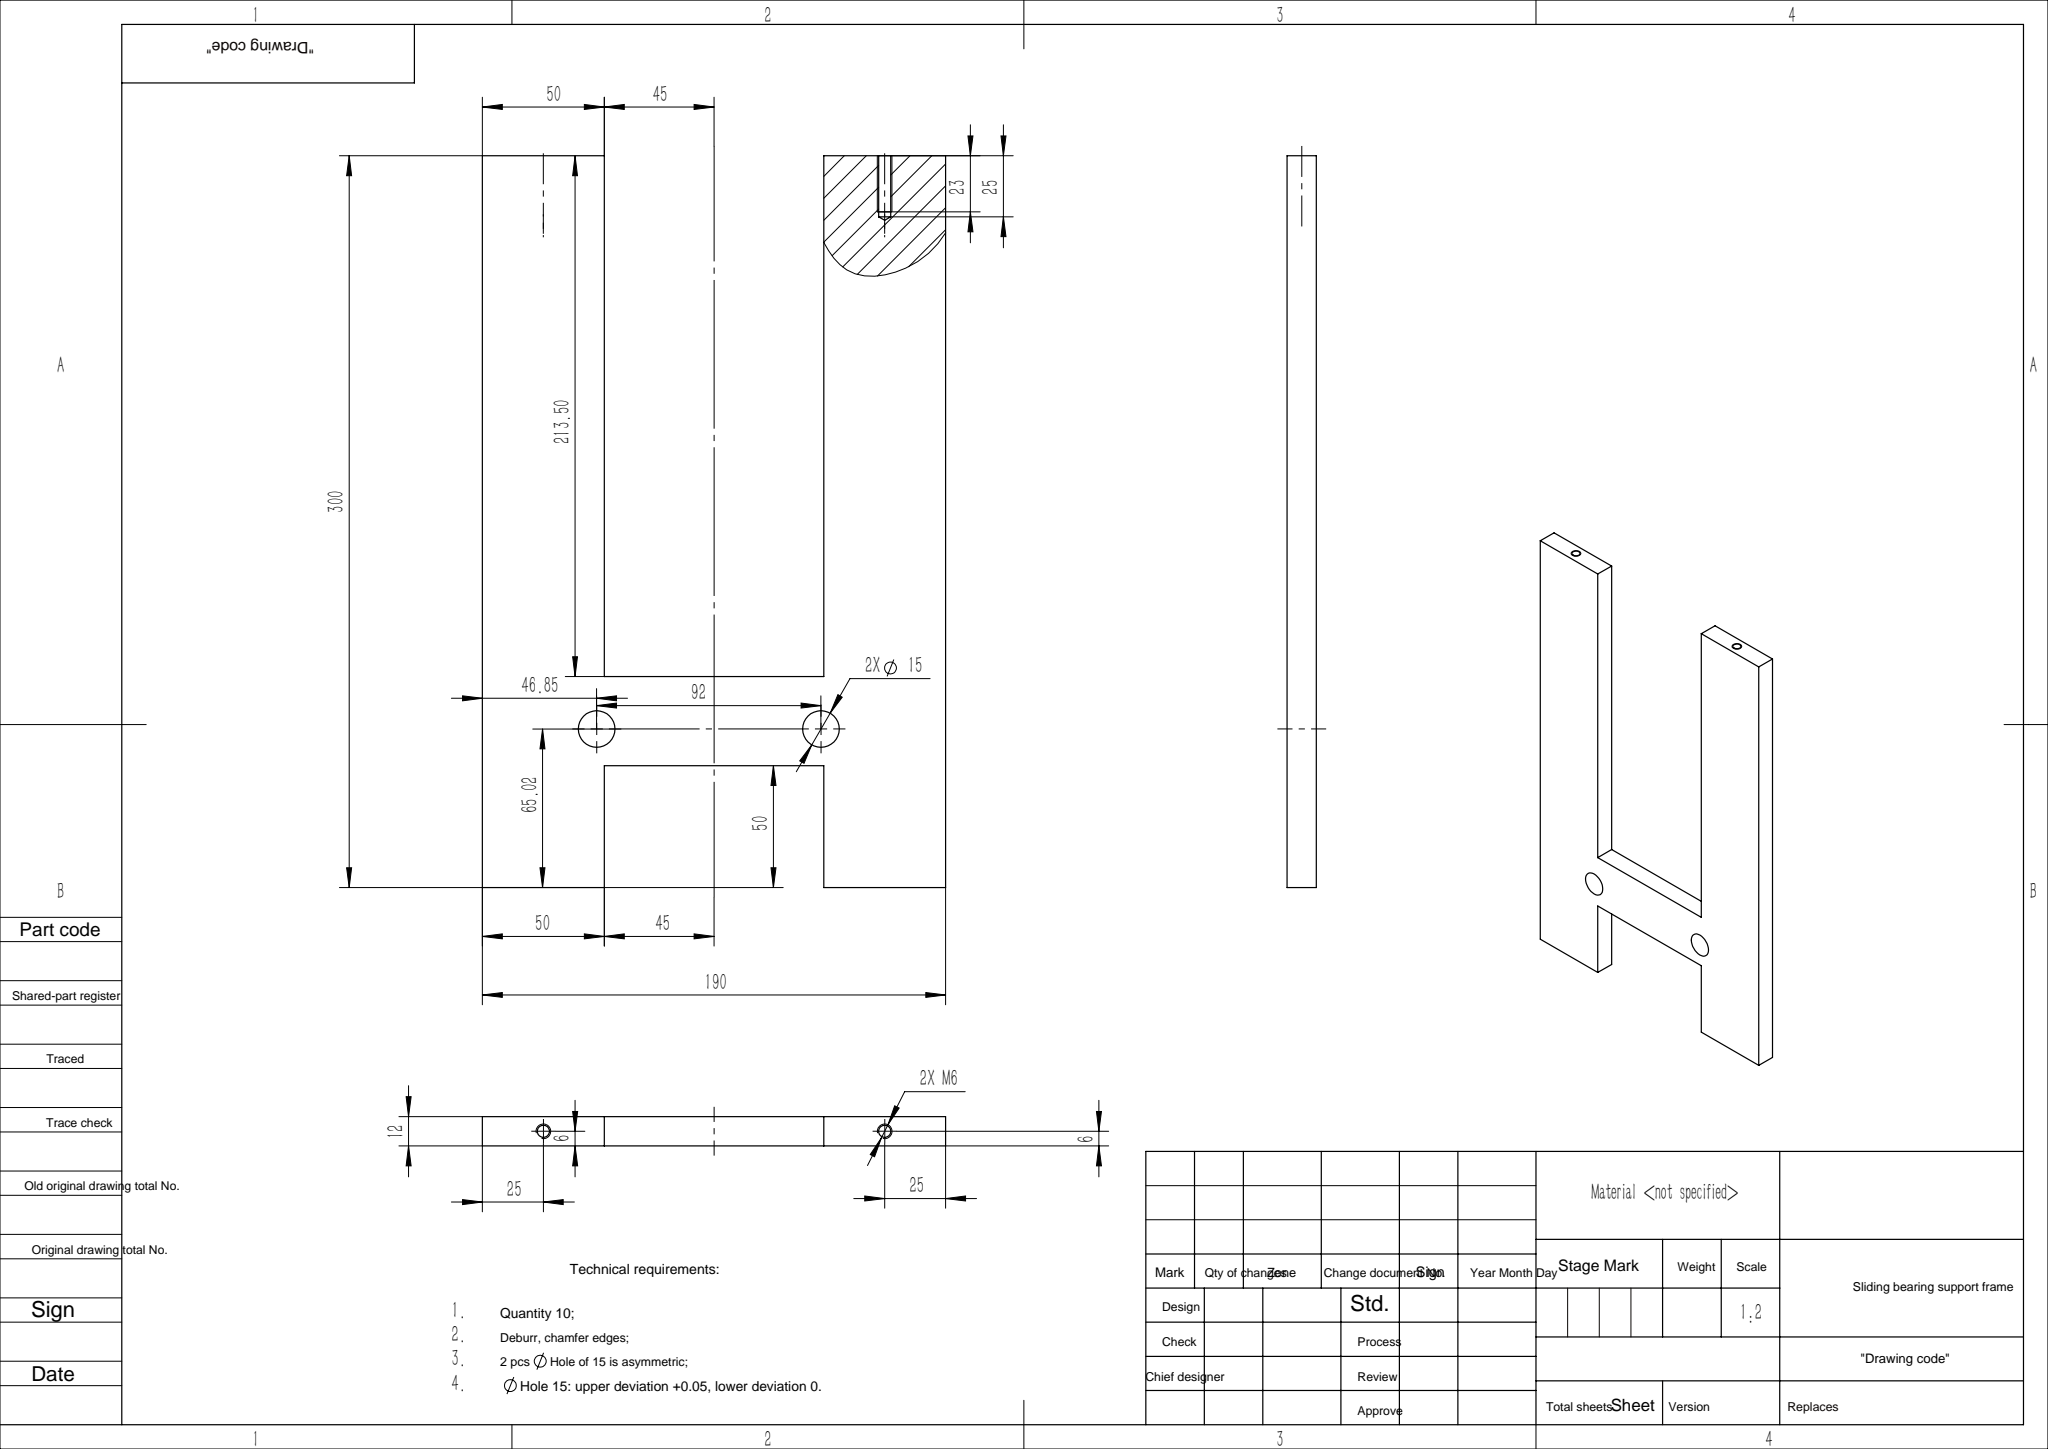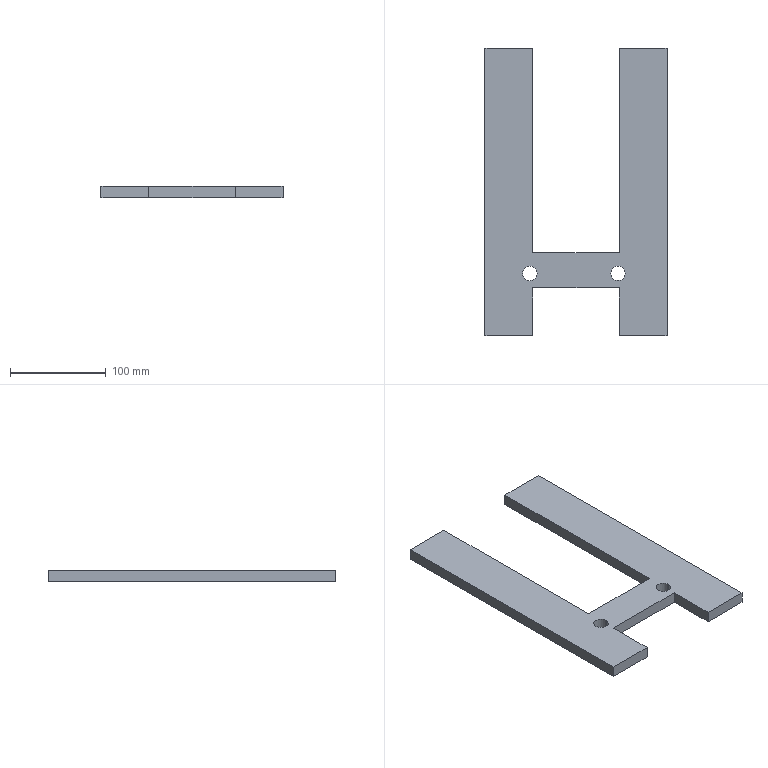Part | SolidWorks | features Extrusion 1, HoleWzd 1 | 1 solid | 26 faces | box 190 x 300 x 12 mm | volume 394178 mm3 | plane 14 | cylinder 8 | cone 4 | commonest cylinder face diameters 5 x4 15 x4
STEP:
#1=CARTESIAN_POINT('',(672.086,1780.,-467.5));
#2=VERTEX_POINT('',#1);
#3=CARTESIAN_POINT('',(672.086,1780.,-462.5));
#4=VERTEX_POINT('',#3);
#5=CARTESIAN_POINT('',(672.086,1780.,-465.));
#6=DIRECTION('',(0.,1.,0.));
#7=DIRECTION('',(0.,0.,1.));
#8=AXIS2_PLACEMENT_3D('',#5,#6,#7);
#9=CIRCLE('',#8,2.5);
#10=EDGE_CURVE('',#2,#4,#9,.T.);
#11=ORIENTED_EDGE('',*,*,#10,.F.);
#12=CARTESIAN_POINT('',(672.086,1805.,-467.5));
#13=VERTEX_POINT('',#12);
#14=CARTESIAN_POINT('',(672.086,1805.,-467.5));
#15=DIRECTION('',(0.,1.,0.));
#16=VECTOR('',#15,1000.);
#17=LINE('',#14,#16);
#18=EDGE_CURVE('',#2,#13,#17,.T.);
#19=ORIENTED_EDGE('',*,*,#18,.T.);
#20=CARTESIAN_POINT('',(672.086,1805.,-462.5));
#21=VERTEX_POINT('',#20);
#22=CARTESIAN_POINT('',(672.086,1805.,-465.));
#23=DIRECTION('',(0.,1.,0.));
#24=DIRECTION('',(0.,0.,1.));
#25=AXIS2_PLACEMENT_3D('',#22,#23,#24);
#26=CIRCLE('',#25,2.5);
#27=EDGE_CURVE('',#13,#21,#26,.T.);
#28=ORIENTED_EDGE('',*,*,#27,.T.);
#29=CARTESIAN_POINT('',(672.086,1805.,-462.5));
#30=DIRECTION('',(0.,1.,0.));
#31=VECTOR('',#30,1000.);
#32=LINE('',#29,#31);
#33=EDGE_CURVE('',#4,#21,#32,.T.);
#34=ORIENTED_EDGE('',*,*,#33,.F.);
#35=EDGE_LOOP('',(#11,#19,#28,#34));
#36=FACE_OUTER_BOUND('',#35,.T.);
#37=CARTESIAN_POINT('',(672.086,1805.,-465.));
#38=DIRECTION('',(0.,1.,0.));
#39=DIRECTION('',(0.,0.,1.));
#40=AXIS2_PLACEMENT_3D('',#37,#38,#39);
#41=CYLINDRICAL_SURFACE('',#40,2.5);
#42=ADVANCED_FACE('',(#36),#41,.F.);
#43=CARTESIAN_POINT('',(672.086,1778.557,-465.));
#44=VERTEX_POINT('',#43);
#45=CARTESIAN_POINT('',(672.086,1780.,-462.5));
#46=DIRECTION('',(0.,0.5,0.866));
#47=VECTOR('',#46,1000.);
#48=LINE('',#45,#47);
#49=EDGE_CURVE('',#44,#4,#48,.T.);
#50=ORIENTED_EDGE('',*,*,#49,.F.);
#51=CARTESIAN_POINT('',(672.086,1780.,-467.5));
#52=DIRECTION('',(0.,0.5,-0.866));
#53=VECTOR('',#52,1000.);
#54=LINE('',#51,#53);
#55=EDGE_CURVE('',#44,#2,#54,.T.);
#56=ORIENTED_EDGE('',*,*,#55,.T.);
#57=ORIENTED_EDGE('',*,*,#10,.T.);
#58=EDGE_LOOP('',(#50,#56,#57));
#59=FACE_OUTER_BOUND('',#58,.T.);
#60=CARTESIAN_POINT('',(672.086,1780.,-465.));
#61=DIRECTION('',(0.,1.,0.));
#62=DIRECTION('',(0.,0.,1.));
#63=AXIS2_PLACEMENT_3D('',#60,#61,#62);
#64=CONICAL_SURFACE('',#63,2.5,1.047);
#65=ADVANCED_FACE('',(#59),#64,.F.);
#66=CARTESIAN_POINT('',(532.086,1780.,-467.5));
#67=VERTEX_POINT('',#66);
#68=CARTESIAN_POINT('',(532.086,1780.,-462.5));
#69=VERTEX_POINT('',#68);
#70=CARTESIAN_POINT('',(532.086,1780.,-465.));
#71=DIRECTION('',(0.,1.,0.));
#72=DIRECTION('',(0.,0.,1.));
#73=AXIS2_PLACEMENT_3D('',#70,#71,#72);
#74=CIRCLE('',#73,2.5);
#75=EDGE_CURVE('',#67,#69,#74,.T.);
#76=ORIENTED_EDGE('',*,*,#75,.F.);
#77=CARTESIAN_POINT('',(532.086,1805.,-467.5));
#78=VERTEX_POINT('',#77);
#79=CARTESIAN_POINT('',(532.086,1805.,-467.5));
#80=DIRECTION('',(0.,1.,0.));
#81=VECTOR('',#80,1000.);
#82=LINE('',#79,#81);
#83=EDGE_CURVE('',#67,#78,#82,.T.);
#84=ORIENTED_EDGE('',*,*,#83,.T.);
#85=CARTESIAN_POINT('',(532.086,1805.,-462.5));
#86=VERTEX_POINT('',#85);
#87=CARTESIAN_POINT('',(532.086,1805.,-465.));
#88=DIRECTION('',(0.,1.,0.));
#89=DIRECTION('',(0.,0.,1.));
#90=AXIS2_PLACEMENT_3D('',#87,#88,#89);
#91=CIRCLE('',#90,2.5);
#92=EDGE_CURVE('',#78,#86,#91,.T.);
#93=ORIENTED_EDGE('',*,*,#92,.T.);
#94=CARTESIAN_POINT('',(532.086,1805.,-462.5));
#95=DIRECTION('',(0.,1.,0.));
#96=VECTOR('',#95,1000.);
#97=LINE('',#94,#96);
#98=EDGE_CURVE('',#69,#86,#97,.T.);
#99=ORIENTED_EDGE('',*,*,#98,.F.);
#100=EDGE_LOOP('',(#76,#84,#93,#99));
#101=FACE_OUTER_BOUND('',#100,.T.);
#102=CARTESIAN_POINT('',(532.086,1805.,-465.));
#103=DIRECTION('',(0.,1.,0.));
#104=DIRECTION('',(0.,0.,1.));
#105=AXIS2_PLACEMENT_3D('',#102,#103,#104);
#106=CYLINDRICAL_SURFACE('',#105,2.5);
#107=ADVANCED_FACE('',(#101),#106,.F.);
#108=CARTESIAN_POINT('',(532.086,1778.557,-465.));
#109=VERTEX_POINT('',#108);
#110=CARTESIAN_POINT('',(532.086,1780.,-462.5));
#111=DIRECTION('',(0.,0.5,0.866));
#112=VECTOR('',#111,1000.);
#113=LINE('',#110,#112);
#114=EDGE_CURVE('',#109,#69,#113,.T.);
#115=ORIENTED_EDGE('',*,*,#114,.F.);
#116=CARTESIAN_POINT('',(532.086,1780.,-467.5));
#117=DIRECTION('',(0.,0.5,-0.866));
#118=VECTOR('',#117,1000.);
#119=LINE('',#116,#118);
#120=EDGE_CURVE('',#109,#67,#119,.T.);
#121=ORIENTED_EDGE('',*,*,#120,.T.);
#122=ORIENTED_EDGE('',*,*,#75,.T.);
#123=EDGE_LOOP('',(#115,#121,#122));
#124=FACE_OUTER_BOUND('',#123,.T.);
#125=CARTESIAN_POINT('',(532.086,1780.,-465.));
#126=DIRECTION('',(0.,1.,0.));
#127=DIRECTION('',(0.,0.,1.));
#128=AXIS2_PLACEMENT_3D('',#125,#126,#127);
#129=CONICAL_SURFACE('',#128,2.5,1.047);
#130=ADVANCED_FACE('',(#124),#129,.F.);
#131=CARTESIAN_POINT('',(653.439,1570.019,-471.));
#132=VERTEX_POINT('',#131);
#133=CARTESIAN_POINT('',(638.439,1570.019,-471.));
#134=VERTEX_POINT('',#133);
#135=CARTESIAN_POINT('',(645.939,1570.019,-471.));
#136=DIRECTION('',(0.,0.,-1.));
#137=DIRECTION('',(-1.,0.,0.));
#138=AXIS2_PLACEMENT_3D('',#135,#136,#137);
#139=CIRCLE('',#138,7.5);
#140=EDGE_CURVE('',#132,#134,#139,.T.);
#141=ORIENTED_EDGE('',*,*,#140,.T.);
#142=CARTESIAN_POINT('',(638.439,1570.019,-459.));
#143=VERTEX_POINT('',#142);
#144=CARTESIAN_POINT('',(638.439,1570.019,-471.));
#145=DIRECTION('',(0.,0.,1.));
#146=VECTOR('',#145,1000.);
#147=LINE('',#144,#146);
#148=EDGE_CURVE('',#134,#143,#147,.T.);
#149=ORIENTED_EDGE('',*,*,#148,.T.);
#150=CARTESIAN_POINT('',(653.439,1570.019,-459.));
#151=VERTEX_POINT('',#150);
#152=CARTESIAN_POINT('',(645.939,1570.019,-459.));
#153=DIRECTION('',(0.,0.,-1.));
#154=DIRECTION('',(-1.,0.,0.));
#155=AXIS2_PLACEMENT_3D('',#152,#153,#154);
#156=CIRCLE('',#155,7.5);
#157=EDGE_CURVE('',#151,#143,#156,.T.);
#158=ORIENTED_EDGE('',*,*,#157,.F.);
#159=CARTESIAN_POINT('',(653.439,1570.019,-471.));
#160=DIRECTION('',(0.,0.,1.));
#161=VECTOR('',#160,1000.);
#162=LINE('',#159,#161);
#163=EDGE_CURVE('',#132,#151,#162,.T.);
#164=ORIENTED_EDGE('',*,*,#163,.F.);
#165=EDGE_LOOP('',(#141,#149,#158,#164));
#166=FACE_OUTER_BOUND('',#165,.T.);
#167=CARTESIAN_POINT('',(645.939,1570.019,-471.));
#168=DIRECTION('',(0.,0.,1.));
#169=DIRECTION('',(1.,0.,0.));
#170=AXIS2_PLACEMENT_3D('',#167,#168,#169);
#171=CYLINDRICAL_SURFACE('',#170,7.5);
#172=ADVANCED_FACE('',(#166),#171,.F.);
#173=CARTESIAN_POINT('',(561.439,1570.019,-471.));
#174=VERTEX_POINT('',#173);
#175=CARTESIAN_POINT('',(546.439,1570.019,-471.));
#176=VERTEX_POINT('',#175);
#177=CARTESIAN_POINT('',(553.939,1570.019,-471.));
#178=DIRECTION('',(0.,0.,-1.));
#179=DIRECTION('',(-1.,0.,0.));
#180=AXIS2_PLACEMENT_3D('',#177,#178,#179);
#181=CIRCLE('',#180,7.5);
#182=EDGE_CURVE('',#174,#176,#181,.T.);
#183=ORIENTED_EDGE('',*,*,#182,.T.);
#184=CARTESIAN_POINT('',(546.439,1570.019,-459.));
#185=VERTEX_POINT('',#184);
#186=CARTESIAN_POINT('',(546.439,1570.019,-471.));
#187=DIRECTION('',(0.,0.,1.));
#188=VECTOR('',#187,1000.);
#189=LINE('',#186,#188);
#190=EDGE_CURVE('',#176,#185,#189,.T.);
#191=ORIENTED_EDGE('',*,*,#190,.T.);
#192=CARTESIAN_POINT('',(561.439,1570.019,-459.));
#193=VERTEX_POINT('',#192);
#194=CARTESIAN_POINT('',(553.939,1570.019,-459.));
#195=DIRECTION('',(0.,0.,-1.));
#196=DIRECTION('',(-1.,0.,0.));
#197=AXIS2_PLACEMENT_3D('',#194,#195,#196);
#198=CIRCLE('',#197,7.5);
#199=EDGE_CURVE('',#193,#185,#198,.T.);
#200=ORIENTED_EDGE('',*,*,#199,.F.);
#201=CARTESIAN_POINT('',(561.439,1570.019,-471.));
#202=DIRECTION('',(0.,0.,1.));
#203=VECTOR('',#202,1000.);
#204=LINE('',#201,#203);
#205=EDGE_CURVE('',#174,#193,#204,.T.);
#206=ORIENTED_EDGE('',*,*,#205,.F.);
#207=EDGE_LOOP('',(#183,#191,#200,#206));
#208=FACE_OUTER_BOUND('',#207,.T.);
#209=CARTESIAN_POINT('',(553.939,1570.019,-471.));
#210=DIRECTION('',(0.,0.,1.));
#211=DIRECTION('',(1.,0.,0.));
#212=AXIS2_PLACEMENT_3D('',#209,#210,#211);
#213=CYLINDRICAL_SURFACE('',#212,7.5);
#214=ADVANCED_FACE('',(#208),#213,.F.);
#215=ORIENTED_EDGE('',*,*,#182,.F.);
#216=CARTESIAN_POINT('',(553.939,1570.019,-471.));
#217=DIRECTION('',(0.,0.,-1.));
#218=DIRECTION('',(-1.,0.,0.));
#219=AXIS2_PLACEMENT_3D('',#216,#217,#218);
#220=CIRCLE('',#219,7.5);
#221=EDGE_CURVE('',#176,#174,#220,.T.);
#222=ORIENTED_EDGE('',*,*,#221,.F.);
#223=EDGE_LOOP('',(#215,#222));
#224=FACE_BOUND('',#223,.T.);
#225=CARTESIAN_POINT('',(507.086,1805.,-471.));
#226=VERTEX_POINT('',#225);
#227=CARTESIAN_POINT('',(557.086,1805.,-471.));
#228=VERTEX_POINT('',#227);
#229=CARTESIAN_POINT('',(557.086,1805.,-471.));
#230=DIRECTION('',(1.,0.,0.));
#231=VECTOR('',#230,1000.);
#232=LINE('',#229,#231);
#233=EDGE_CURVE('',#226,#228,#232,.T.);
#234=ORIENTED_EDGE('',*,*,#233,.T.);
#235=CARTESIAN_POINT('',(557.086,1591.5,-471.));
#236=VERTEX_POINT('',#235);
#237=CARTESIAN_POINT('',(557.086,1805.,-471.));
#238=DIRECTION('',(0.,-1.,0.));
#239=VECTOR('',#238,1000.);
#240=LINE('',#237,#239);
#241=EDGE_CURVE('',#228,#236,#240,.T.);
#242=ORIENTED_EDGE('',*,*,#241,.T.);
#243=CARTESIAN_POINT('',(647.086,1591.5,-471.));
#244=VERTEX_POINT('',#243);
#245=CARTESIAN_POINT('',(557.086,1591.5,-471.));
#246=DIRECTION('',(1.,0.,0.));
#247=VECTOR('',#246,1000.);
#248=LINE('',#245,#247);
#249=EDGE_CURVE('',#236,#244,#248,.T.);
#250=ORIENTED_EDGE('',*,*,#249,.T.);
#251=CARTESIAN_POINT('',(647.086,1805.,-471.));
#252=VERTEX_POINT('',#251);
#253=CARTESIAN_POINT('',(647.086,1805.,-471.));
#254=DIRECTION('',(0.,1.,0.));
#255=VECTOR('',#254,1000.);
#256=LINE('',#253,#255);
#257=EDGE_CURVE('',#244,#252,#256,.T.);
#258=ORIENTED_EDGE('',*,*,#257,.T.);
#259=CARTESIAN_POINT('',(697.086,1805.,-471.));
#260=VERTEX_POINT('',#259);
#261=CARTESIAN_POINT('',(647.086,1805.,-471.));
#262=DIRECTION('',(1.,0.,0.));
#263=VECTOR('',#262,1000.);
#264=LINE('',#261,#263);
#265=EDGE_CURVE('',#252,#260,#264,.T.);
#266=ORIENTED_EDGE('',*,*,#265,.T.);
#267=CARTESIAN_POINT('',(697.086,1505.,-471.));
#268=VERTEX_POINT('',#267);
#269=CARTESIAN_POINT('',(697.086,1805.,-471.));
#270=DIRECTION('',(0.,-1.,0.));
#271=VECTOR('',#270,1000.);
#272=LINE('',#269,#271);
#273=EDGE_CURVE('',#260,#268,#272,.T.);
#274=ORIENTED_EDGE('',*,*,#273,.T.);
#275=CARTESIAN_POINT('',(647.086,1505.,-471.));
#276=VERTEX_POINT('',#275);
#277=CARTESIAN_POINT('',(697.086,1505.,-471.));
#278=DIRECTION('',(-1.,0.,0.));
#279=VECTOR('',#278,1000.);
#280=LINE('',#277,#279);
#281=EDGE_CURVE('',#268,#276,#280,.T.);
#282=ORIENTED_EDGE('',*,*,#281,.T.);
#283=CARTESIAN_POINT('',(647.086,1555.,-471.));
#284=VERTEX_POINT('',#283);
#285=CARTESIAN_POINT('',(647.086,1555.,-471.));
#286=DIRECTION('',(0.,1.,0.));
#287=VECTOR('',#286,1000.);
#288=LINE('',#285,#287);
#289=EDGE_CURVE('',#276,#284,#288,.T.);
#290=ORIENTED_EDGE('',*,*,#289,.T.);
#291=CARTESIAN_POINT('',(557.086,1555.,-471.));
#292=VERTEX_POINT('',#291);
#293=CARTESIAN_POINT('',(647.086,1555.,-471.));
#294=DIRECTION('',(-1.,0.,0.));
#295=VECTOR('',#294,1000.);
#296=LINE('',#293,#295);
#297=EDGE_CURVE('',#284,#292,#296,.T.);
#298=ORIENTED_EDGE('',*,*,#297,.T.);
#299=CARTESIAN_POINT('',(557.086,1505.,-471.));
#300=VERTEX_POINT('',#299);
#301=CARTESIAN_POINT('',(557.086,1555.,-471.));
#302=DIRECTION('',(0.,-1.,0.));
#303=VECTOR('',#302,1000.);
#304=LINE('',#301,#303);
#305=EDGE_CURVE('',#292,#300,#304,.T.);
#306=ORIENTED_EDGE('',*,*,#305,.T.);
#307=CARTESIAN_POINT('',(507.086,1505.,-471.));
#308=VERTEX_POINT('',#307);
#309=CARTESIAN_POINT('',(507.086,1505.,-471.));
#310=DIRECTION('',(-1.,0.,0.));
#311=VECTOR('',#310,1000.);
#312=LINE('',#309,#311);
#313=EDGE_CURVE('',#300,#308,#312,.T.);
#314=ORIENTED_EDGE('',*,*,#313,.T.);
#315=CARTESIAN_POINT('',(507.086,1805.,-471.));
#316=DIRECTION('',(0.,1.,0.));
#317=VECTOR('',#316,1000.);
#318=LINE('',#315,#317);
#319=EDGE_CURVE('',#308,#226,#318,.T.);
#320=ORIENTED_EDGE('',*,*,#319,.T.);
#321=EDGE_LOOP('',(#234,#242,#250,#258,#266,#274,#282,#290,#298,#306,#314,#320));
#322=FACE_OUTER_BOUND('',#321,.T.);
#323=ORIENTED_EDGE('',*,*,#140,.F.);
#324=CARTESIAN_POINT('',(645.939,1570.019,-471.));
#325=DIRECTION('',(0.,0.,-1.));
#326=DIRECTION('',(-1.,0.,0.));
#327=AXIS2_PLACEMENT_3D('',#324,#325,#326);
#328=CIRCLE('',#327,7.5);
#329=EDGE_CURVE('',#134,#132,#328,.T.);
#330=ORIENTED_EDGE('',*,*,#329,.F.);
#331=EDGE_LOOP('',(#323,#330));
#332=FACE_BOUND('',#331,.T.);
#333=CARTESIAN_POINT('',(0.,0.,-471.));
#334=DIRECTION('',(0.,0.,1.));
#335=DIRECTION('',(1.,0.,0.));
#336=AXIS2_PLACEMENT_3D('',#333,#334,#335);
#337=PLANE('',#336);
#338=ADVANCED_FACE('',(#224,#322,#332),#337,.F.);
#339=ORIENTED_EDGE('',*,*,#199,.T.);
#340=CARTESIAN_POINT('',(553.939,1570.019,-459.));
#341=DIRECTION('',(0.,0.,-1.));
#342=DIRECTION('',(-1.,0.,0.));
#343=AXIS2_PLACEMENT_3D('',#340,#341,#342);
#344=CIRCLE('',#343,7.5);
#345=EDGE_CURVE('',#185,#193,#344,.T.);
#346=ORIENTED_EDGE('',*,*,#345,.T.);
#347=EDGE_LOOP('',(#339,#346));
#348=FACE_BOUND('',#347,.T.);
#349=CARTESIAN_POINT('',(507.086,1805.,-459.));
#350=VERTEX_POINT('',#349);
#351=CARTESIAN_POINT('',(557.086,1805.,-459.));
#352=VERTEX_POINT('',#351);
#353=CARTESIAN_POINT('',(557.086,1805.,-459.));
#354=DIRECTION('',(1.,0.,0.));
#355=VECTOR('',#354,1000.);
#356=LINE('',#353,#355);
#357=EDGE_CURVE('',#350,#352,#356,.T.);
#358=ORIENTED_EDGE('',*,*,#357,.F.);
#359=CARTESIAN_POINT('',(507.086,1505.,-459.));
#360=VERTEX_POINT('',#359);
#361=CARTESIAN_POINT('',(507.086,1805.,-459.));
#362=DIRECTION('',(0.,1.,0.));
#363=VECTOR('',#362,1000.);
#364=LINE('',#361,#363);
#365=EDGE_CURVE('',#360,#350,#364,.T.);
#366=ORIENTED_EDGE('',*,*,#365,.F.);
#367=CARTESIAN_POINT('',(557.086,1505.,-459.));
#368=VERTEX_POINT('',#367);
#369=CARTESIAN_POINT('',(507.086,1505.,-459.));
#370=DIRECTION('',(-1.,0.,0.));
#371=VECTOR('',#370,1000.);
#372=LINE('',#369,#371);
#373=EDGE_CURVE('',#368,#360,#372,.T.);
#374=ORIENTED_EDGE('',*,*,#373,.F.);
#375=CARTESIAN_POINT('',(557.086,1555.,-459.));
#376=VERTEX_POINT('',#375);
#377=CARTESIAN_POINT('',(557.086,1555.,-459.));
#378=DIRECTION('',(0.,-1.,0.));
#379=VECTOR('',#378,1000.);
#380=LINE('',#377,#379);
#381=EDGE_CURVE('',#376,#368,#380,.T.);
#382=ORIENTED_EDGE('',*,*,#381,.F.);
#383=CARTESIAN_POINT('',(647.086,1555.,-459.));
#384=VERTEX_POINT('',#383);
#385=CARTESIAN_POINT('',(647.086,1555.,-459.));
#386=DIRECTION('',(-1.,0.,0.));
#387=VECTOR('',#386,1000.);
#388=LINE('',#385,#387);
#389=EDGE_CURVE('',#384,#376,#388,.T.);
#390=ORIENTED_EDGE('',*,*,#389,.F.);
#391=CARTESIAN_POINT('',(647.086,1505.,-459.));
#392=VERTEX_POINT('',#391);
#393=CARTESIAN_POINT('',(647.086,1555.,-459.));
#394=DIRECTION('',(0.,1.,0.));
#395=VECTOR('',#394,1000.);
#396=LINE('',#393,#395);
#397=EDGE_CURVE('',#392,#384,#396,.T.);
#398=ORIENTED_EDGE('',*,*,#397,.F.);
#399=CARTESIAN_POINT('',(697.086,1505.,-459.));
#400=VERTEX_POINT('',#399);
#401=CARTESIAN_POINT('',(697.086,1505.,-459.));
#402=DIRECTION('',(-1.,0.,0.));
#403=VECTOR('',#402,1000.);
#404=LINE('',#401,#403);
#405=EDGE_CURVE('',#400,#392,#404,.T.);
#406=ORIENTED_EDGE('',*,*,#405,.F.);
#407=CARTESIAN_POINT('',(697.086,1805.,-459.));
#408=VERTEX_POINT('',#407);
#409=CARTESIAN_POINT('',(697.086,1805.,-459.));
#410=DIRECTION('',(0.,-1.,0.));
#411=VECTOR('',#410,1000.);
#412=LINE('',#409,#411);
#413=EDGE_CURVE('',#408,#400,#412,.T.);
#414=ORIENTED_EDGE('',*,*,#413,.F.);
#415=CARTESIAN_POINT('',(647.086,1805.,-459.));
#416=VERTEX_POINT('',#415);
#417=CARTESIAN_POINT('',(647.086,1805.,-459.));
#418=DIRECTION('',(1.,0.,0.));
#419=VECTOR('',#418,1000.);
#420=LINE('',#417,#419);
#421=EDGE_CURVE('',#416,#408,#420,.T.);
#422=ORIENTED_EDGE('',*,*,#421,.F.);
#423=CARTESIAN_POINT('',(647.086,1591.5,-459.));
#424=VERTEX_POINT('',#423);
#425=CARTESIAN_POINT('',(647.086,1805.,-459.));
#426=DIRECTION('',(0.,1.,0.));
#427=VECTOR('',#426,1000.);
#428=LINE('',#425,#427);
#429=EDGE_CURVE('',#424,#416,#428,.T.);
#430=ORIENTED_EDGE('',*,*,#429,.F.);
#431=CARTESIAN_POINT('',(557.086,1591.5,-459.));
#432=VERTEX_POINT('',#431);
#433=CARTESIAN_POINT('',(557.086,1591.5,-459.));
#434=DIRECTION('',(1.,0.,0.));
#435=VECTOR('',#434,1000.);
#436=LINE('',#433,#435);
#437=EDGE_CURVE('',#432,#424,#436,.T.);
#438=ORIENTED_EDGE('',*,*,#437,.F.);
#439=CARTESIAN_POINT('',(557.086,1805.,-459.));
#440=DIRECTION('',(0.,-1.,0.));
#441=VECTOR('',#440,1000.);
#442=LINE('',#439,#441);
#443=EDGE_CURVE('',#352,#432,#442,.T.);
#444=ORIENTED_EDGE('',*,*,#443,.F.);
#445=EDGE_LOOP('',(#358,#366,#374,#382,#390,#398,#406,#414,#422,#430,#438,#444));
#446=FACE_OUTER_BOUND('',#445,.T.);
#447=ORIENTED_EDGE('',*,*,#157,.T.);
#448=CARTESIAN_POINT('',(645.939,1570.019,-459.));
#449=DIRECTION('',(0.,0.,-1.));
#450=DIRECTION('',(-1.,0.,0.));
#451=AXIS2_PLACEMENT_3D('',#448,#449,#450);
#452=CIRCLE('',#451,7.5);
#453=EDGE_CURVE('',#143,#151,#452,.T.);
#454=ORIENTED_EDGE('',*,*,#453,.T.);
#455=EDGE_LOOP('',(#447,#454));
#456=FACE_BOUND('',#455,.T.);
#457=CARTESIAN_POINT('',(0.,0.,-459.));
#458=DIRECTION('',(0.,0.,1.));
#459=DIRECTION('',(1.,0.,0.));
#460=AXIS2_PLACEMENT_3D('',#457,#458,#459);
#461=PLANE('',#460);
#462=ADVANCED_FACE('',(#348,#446,#456),#461,.T.);
#463=CARTESIAN_POINT('',(532.086,1805.,-465.));
#464=DIRECTION('',(0.,1.,0.));
#465=DIRECTION('',(0.,0.,1.));
#466=AXIS2_PLACEMENT_3D('',#463,#464,#465);
#467=CIRCLE('',#466,2.5);
#468=EDGE_CURVE('',#86,#78,#467,.T.);
#469=ORIENTED_EDGE('',*,*,#468,.F.);
#470=ORIENTED_EDGE('',*,*,#92,.F.);
#471=EDGE_LOOP('',(#469,#470));
#472=FACE_BOUND('',#471,.T.);
#473=ORIENTED_EDGE('',*,*,#357,.T.);
#474=CARTESIAN_POINT('',(557.086,1805.,-471.));
#475=DIRECTION('',(0.,0.,1.));
#476=VECTOR('',#475,1000.);
#477=LINE('',#474,#476);
#478=EDGE_CURVE('',#228,#352,#477,.T.);
#479=ORIENTED_EDGE('',*,*,#478,.F.);
#480=ORIENTED_EDGE('',*,*,#233,.F.);
#481=CARTESIAN_POINT('',(507.086,1805.,-471.));
#482=DIRECTION('',(0.,0.,1.));
#483=VECTOR('',#482,1000.);
#484=LINE('',#481,#483);
#485=EDGE_CURVE('',#226,#350,#484,.T.);
#486=ORIENTED_EDGE('',*,*,#485,.T.);
#487=EDGE_LOOP('',(#473,#479,#480,#486));
#488=FACE_OUTER_BOUND('',#487,.T.);
#489=CARTESIAN_POINT('',(557.086,1805.,-471.));
#490=DIRECTION('',(0.,-1.,0.));
#491=DIRECTION('',(1.,0.,0.));
#492=AXIS2_PLACEMENT_3D('',#489,#490,#491);
#493=PLANE('',#492);
#494=ADVANCED_FACE('',(#472,#488),#493,.F.);
#495=ORIENTED_EDGE('',*,*,#443,.T.);
#496=CARTESIAN_POINT('',(557.086,1591.5,-471.));
#497=DIRECTION('',(0.,0.,1.));
#498=VECTOR('',#497,1000.);
#499=LINE('',#496,#498);
#500=EDGE_CURVE('',#236,#432,#499,.T.);
#501=ORIENTED_EDGE('',*,*,#500,.F.);
#502=ORIENTED_EDGE('',*,*,#241,.F.);
#503=ORIENTED_EDGE('',*,*,#478,.T.);
#504=EDGE_LOOP('',(#495,#501,#502,#503));
#505=FACE_OUTER_BOUND('',#504,.T.);
#506=CARTESIAN_POINT('',(557.086,1805.,-471.));
#507=DIRECTION('',(-1.,0.,0.));
#508=DIRECTION('',(0.,0.,1.));
#509=AXIS2_PLACEMENT_3D('',#506,#507,#508);
#510=PLANE('',#509);
#511=ADVANCED_FACE('',(#505),#510,.F.);
#512=ORIENTED_EDGE('',*,*,#437,.T.);
#513=CARTESIAN_POINT('',(647.086,1591.5,-471.));
#514=DIRECTION('',(0.,0.,1.));
#515=VECTOR('',#514,1000.);
#516=LINE('',#513,#515);
#517=EDGE_CURVE('',#244,#424,#516,.T.);
#518=ORIENTED_EDGE('',*,*,#517,.F.);
#519=ORIENTED_EDGE('',*,*,#249,.F.);
#520=ORIENTED_EDGE('',*,*,#500,.T.);
#521=EDGE_LOOP('',(#512,#518,#519,#520));
#522=FACE_OUTER_BOUND('',#521,.T.);
#523=CARTESIAN_POINT('',(557.086,1591.5,-471.));
#524=DIRECTION('',(0.,-1.,0.));
#525=DIRECTION('',(0.,0.,-1.));
#526=AXIS2_PLACEMENT_3D('',#523,#524,#525);
#527=PLANE('',#526);
#528=ADVANCED_FACE('',(#522),#527,.F.);
#529=ORIENTED_EDGE('',*,*,#429,.T.);
#530=CARTESIAN_POINT('',(647.086,1805.,-471.));
#531=DIRECTION('',(0.,0.,1.));
#532=VECTOR('',#531,1000.);
#533=LINE('',#530,#532);
#534=EDGE_CURVE('',#252,#416,#533,.T.);
#535=ORIENTED_EDGE('',*,*,#534,.F.);
#536=ORIENTED_EDGE('',*,*,#257,.F.);
#537=ORIENTED_EDGE('',*,*,#517,.T.);
#538=EDGE_LOOP('',(#529,#535,#536,#537));
#539=FACE_OUTER_BOUND('',#538,.T.);
#540=CARTESIAN_POINT('',(647.086,1805.,-471.));
#541=DIRECTION('',(1.,0.,0.));
#542=DIRECTION('',(0.,0.,-1.));
#543=AXIS2_PLACEMENT_3D('',#540,#541,#542);
#544=PLANE('',#543);
#545=ADVANCED_FACE('',(#539),#544,.F.);
#546=CARTESIAN_POINT('',(672.086,1805.,-465.));
#547=DIRECTION('',(0.,1.,0.));
#548=DIRECTION('',(0.,0.,1.));
#549=AXIS2_PLACEMENT_3D('',#546,#547,#548);
#550=CIRCLE('',#549,2.5);
#551=EDGE_CURVE('',#21,#13,#550,.T.);
#552=ORIENTED_EDGE('',*,*,#551,.F.);
#553=ORIENTED_EDGE('',*,*,#27,.F.);
#554=EDGE_LOOP('',(#552,#553));
#555=FACE_BOUND('',#554,.T.);
#556=ORIENTED_EDGE('',*,*,#421,.T.);
#557=CARTESIAN_POINT('',(697.086,1805.,-471.));
#558=DIRECTION('',(0.,0.,1.));
#559=VECTOR('',#558,1000.);
#560=LINE('',#557,#559);
#561=EDGE_CURVE('',#260,#408,#560,.T.);
#562=ORIENTED_EDGE('',*,*,#561,.F.);
#563=ORIENTED_EDGE('',*,*,#265,.F.);
#564=ORIENTED_EDGE('',*,*,#534,.T.);
#565=EDGE_LOOP('',(#556,#562,#563,#564));
#566=FACE_OUTER_BOUND('',#565,.T.);
#567=CARTESIAN_POINT('',(647.086,1805.,-471.));
#568=DIRECTION('',(0.,-1.,0.));
#569=DIRECTION('',(1.,0.,0.));
#570=AXIS2_PLACEMENT_3D('',#567,#568,#569);
#571=PLANE('',#570);
#572=ADVANCED_FACE('',(#555,#566),#571,.F.);
#573=ORIENTED_EDGE('',*,*,#413,.T.);
#574=CARTESIAN_POINT('',(697.086,1505.,-471.));
#575=DIRECTION('',(0.,0.,1.));
#576=VECTOR('',#575,1000.);
#577=LINE('',#574,#576);
#578=EDGE_CURVE('',#268,#400,#577,.T.);
#579=ORIENTED_EDGE('',*,*,#578,.F.);
#580=ORIENTED_EDGE('',*,*,#273,.F.);
#581=ORIENTED_EDGE('',*,*,#561,.T.);
#582=EDGE_LOOP('',(#573,#579,#580,#581));
#583=FACE_OUTER_BOUND('',#582,.T.);
#584=CARTESIAN_POINT('',(697.086,1805.,-471.));
#585=DIRECTION('',(-1.,0.,0.));
#586=DIRECTION('',(0.,-1.,0.));
#587=AXIS2_PLACEMENT_3D('',#584,#585,#586);
#588=PLANE('',#587);
#589=ADVANCED_FACE('',(#583),#588,.F.);
#590=ORIENTED_EDGE('',*,*,#405,.T.);
#591=CARTESIAN_POINT('',(647.086,1505.,-471.));
#592=DIRECTION('',(0.,0.,1.));
#593=VECTOR('',#592,1000.);
#594=LINE('',#591,#593);
#595=EDGE_CURVE('',#276,#392,#594,.T.);
#596=ORIENTED_EDGE('',*,*,#595,.F.);
#597=ORIENTED_EDGE('',*,*,#281,.F.);
#598=ORIENTED_EDGE('',*,*,#578,.T.);
#599=EDGE_LOOP('',(#590,#596,#597,#598));
#600=FACE_OUTER_BOUND('',#599,.T.);
#601=CARTESIAN_POINT('',(697.086,1505.,-471.));
#602=DIRECTION('',(0.,1.,0.));
#603=DIRECTION('',(0.,0.,1.));
#604=AXIS2_PLACEMENT_3D('',#601,#602,#603);
#605=PLANE('',#604);
#606=ADVANCED_FACE('',(#600),#605,.F.);
#607=ORIENTED_EDGE('',*,*,#397,.T.);
#608=CARTESIAN_POINT('',(647.086,1555.,-471.));
#609=DIRECTION('',(0.,0.,1.));
#610=VECTOR('',#609,1000.);
#611=LINE('',#608,#610);
#612=EDGE_CURVE('',#284,#384,#611,.T.);
#613=ORIENTED_EDGE('',*,*,#612,.F.);
#614=ORIENTED_EDGE('',*,*,#289,.F.);
#615=ORIENTED_EDGE('',*,*,#595,.T.);
#616=EDGE_LOOP('',(#607,#613,#614,#615));
#617=FACE_OUTER_BOUND('',#616,.T.);
#618=CARTESIAN_POINT('',(647.086,1555.,-471.));
#619=DIRECTION('',(1.,0.,0.));
#620=DIRECTION('',(0.,1.,0.));
#621=AXIS2_PLACEMENT_3D('',#618,#619,#620);
#622=PLANE('',#621);
#623=ADVANCED_FACE('',(#617),#622,.F.);
#624=ORIENTED_EDGE('',*,*,#389,.T.);
#625=CARTESIAN_POINT('',(557.086,1555.,-471.));
#626=DIRECTION('',(0.,0.,1.));
#627=VECTOR('',#626,1000.);
#628=LINE('',#625,#627);
#629=EDGE_CURVE('',#292,#376,#628,.T.);
#630=ORIENTED_EDGE('',*,*,#629,.F.);
#631=ORIENTED_EDGE('',*,*,#297,.F.);
#632=ORIENTED_EDGE('',*,*,#612,.T.);
#633=EDGE_LOOP('',(#624,#630,#631,#632));
#634=FACE_OUTER_BOUND('',#633,.T.);
#635=CARTESIAN_POINT('',(647.086,1555.,-471.));
#636=DIRECTION('',(0.,1.,0.));
#637=DIRECTION('',(0.,0.,1.));
#638=AXIS2_PLACEMENT_3D('',#635,#636,#637);
#639=PLANE('',#638);
#640=ADVANCED_FACE('',(#634),#639,.F.);
#641=ORIENTED_EDGE('',*,*,#381,.T.);
#642=CARTESIAN_POINT('',(557.086,1505.,-471.));
#643=DIRECTION('',(0.,0.,1.));
#644=VECTOR('',#643,1000.);
#645=LINE('',#642,#644);
#646=EDGE_CURVE('',#300,#368,#645,.T.);
#647=ORIENTED_EDGE('',*,*,#646,.F.);
#648=ORIENTED_EDGE('',*,*,#305,.F.);
#649=ORIENTED_EDGE('',*,*,#629,.T.);
#650=EDGE_LOOP('',(#641,#647,#648,#649));
#651=FACE_OUTER_BOUND('',#650,.T.);
#652=CARTESIAN_POINT('',(557.086,1555.,-471.));
#653=DIRECTION('',(-1.,0.,0.));
#654=DIRECTION('',(0.,-1.,0.));
#655=AXIS2_PLACEMENT_3D('',#652,#653,#654);
#656=PLANE('',#655);
#657=ADVANCED_FACE('',(#651),#656,.F.);
#658=ORIENTED_EDGE('',*,*,#373,.T.);
#659=CARTESIAN_POINT('',(507.086,1505.,-471.));
#660=DIRECTION('',(0.,0.,1.));
#661=VECTOR('',#660,1000.);
#662=LINE('',#659,#661);
#663=EDGE_CURVE('',#308,#360,#662,.T.);
#664=ORIENTED_EDGE('',*,*,#663,.F.);
#665=ORIENTED_EDGE('',*,*,#313,.F.);
#666=ORIENTED_EDGE('',*,*,#646,.T.);
#667=EDGE_LOOP('',(#658,#664,#665,#666));
#668=FACE_OUTER_BOUND('',#667,.T.);
#669=CARTESIAN_POINT('',(507.086,1505.,-471.));
#670=DIRECTION('',(0.,1.,0.));
#671=DIRECTION('',(0.,0.,1.));
#672=AXIS2_PLACEMENT_3D('',#669,#670,#671);
#673=PLANE('',#672);
#674=ADVANCED_FACE('',(#668),#673,.F.);
#675=ORIENTED_EDGE('',*,*,#365,.T.);
#676=ORIENTED_EDGE('',*,*,#485,.F.);
#677=ORIENTED_EDGE('',*,*,#319,.F.);
#678=ORIENTED_EDGE('',*,*,#663,.T.);
#679=EDGE_LOOP('',(#675,#676,#677,#678));
#680=FACE_OUTER_BOUND('',#679,.T.);
#681=CARTESIAN_POINT('',(507.086,1805.,-471.));
#682=DIRECTION('',(1.,0.,0.));
#683=DIRECTION('',(0.,1.,0.));
#684=AXIS2_PLACEMENT_3D('',#681,#682,#683);
#685=PLANE('',#684);
#686=ADVANCED_FACE('',(#680),#685,.F.);
#687=ORIENTED_EDGE('',*,*,#190,.F.);
#688=ORIENTED_EDGE('',*,*,#221,.T.);
#689=ORIENTED_EDGE('',*,*,#205,.T.);
#690=ORIENTED_EDGE('',*,*,#345,.F.);
#691=EDGE_LOOP('',(#687,#688,#689,#690));
#692=FACE_OUTER_BOUND('',#691,.T.);
#693=CARTESIAN_POINT('',(553.939,1570.019,-471.));
#694=DIRECTION('',(0.,0.,1.));
#695=DIRECTION('',(1.,0.,0.));
#696=AXIS2_PLACEMENT_3D('',#693,#694,#695);
#697=CYLINDRICAL_SURFACE('',#696,7.5);
#698=ADVANCED_FACE('',(#692),#697,.F.);
#699=ORIENTED_EDGE('',*,*,#148,.F.);
#700=ORIENTED_EDGE('',*,*,#329,.T.);
#701=ORIENTED_EDGE('',*,*,#163,.T.);
#702=ORIENTED_EDGE('',*,*,#453,.F.);
#703=EDGE_LOOP('',(#699,#700,#701,#702));
#704=FACE_OUTER_BOUND('',#703,.T.);
#705=CARTESIAN_POINT('',(645.939,1570.019,-471.));
#706=DIRECTION('',(0.,0.,1.));
#707=DIRECTION('',(1.,0.,0.));
#708=AXIS2_PLACEMENT_3D('',#705,#706,#707);
#709=CYLINDRICAL_SURFACE('',#708,7.5);
#710=ADVANCED_FACE('',(#704),#709,.F.);
#711=ORIENTED_EDGE('',*,*,#120,.F.);
#712=ORIENTED_EDGE('',*,*,#114,.T.);
#713=CARTESIAN_POINT('',(532.086,1780.,-465.));
#714=DIRECTION('',(0.,1.,0.));
#715=DIRECTION('',(0.,0.,1.));
#716=AXIS2_PLACEMENT_3D('',#713,#714,#715);
#717=CIRCLE('',#716,2.5);
#718=EDGE_CURVE('',#69,#67,#717,.T.);
#719=ORIENTED_EDGE('',*,*,#718,.T.);
#720=EDGE_LOOP('',(#711,#712,#719));
#721=FACE_OUTER_BOUND('',#720,.T.);
#722=CARTESIAN_POINT('',(532.086,1780.,-465.));
#723=DIRECTION('',(0.,1.,0.));
#724=DIRECTION('',(0.,0.,1.));
#725=AXIS2_PLACEMENT_3D('',#722,#723,#724);
#726=CONICAL_SURFACE('',#725,2.5,1.047);
#727=ADVANCED_FACE('',(#721),#726,.F.);
#728=ORIENTED_EDGE('',*,*,#83,.F.);
#729=ORIENTED_EDGE('',*,*,#718,.F.);
#730=ORIENTED_EDGE('',*,*,#98,.T.);
#731=ORIENTED_EDGE('',*,*,#468,.T.);
#732=EDGE_LOOP('',(#728,#729,#730,#731));
#733=FACE_OUTER_BOUND('',#732,.T.);
#734=CARTESIAN_POINT('',(532.086,1805.,-465.));
#735=DIRECTION('',(0.,1.,0.));
#736=DIRECTION('',(0.,0.,1.));
#737=AXIS2_PLACEMENT_3D('',#734,#735,#736);
#738=CYLINDRICAL_SURFACE('',#737,2.5);
#739=ADVANCED_FACE('',(#733),#738,.F.);
#740=ORIENTED_EDGE('',*,*,#55,.F.);
#741=ORIENTED_EDGE('',*,*,#49,.T.);
#742=CARTESIAN_POINT('',(672.086,1780.,-465.));
#743=DIRECTION('',(0.,1.,0.));
#744=DIRECTION('',(0.,0.,1.));
#745=AXIS2_PLACEMENT_3D('',#742,#743,#744);
#746=CIRCLE('',#745,2.5);
#747=EDGE_CURVE('',#4,#2,#746,.T.);
#748=ORIENTED_EDGE('',*,*,#747,.T.);
#749=EDGE_LOOP('',(#740,#741,#748));
#750=FACE_OUTER_BOUND('',#749,.T.);
#751=CARTESIAN_POINT('',(672.086,1780.,-465.));
#752=DIRECTION('',(0.,1.,0.));
#753=DIRECTION('',(0.,0.,1.));
#754=AXIS2_PLACEMENT_3D('',#751,#752,#753);
#755=CONICAL_SURFACE('',#754,2.5,1.047);
#756=ADVANCED_FACE('',(#750),#755,.F.);
#757=ORIENTED_EDGE('',*,*,#18,.F.);
#758=ORIENTED_EDGE('',*,*,#747,.F.);
#759=ORIENTED_EDGE('',*,*,#33,.T.);
#760=ORIENTED_EDGE('',*,*,#551,.T.);
#761=EDGE_LOOP('',(#757,#758,#759,#760));
#762=FACE_OUTER_BOUND('',#761,.T.);
#763=CARTESIAN_POINT('',(672.086,1805.,-465.));
#764=DIRECTION('',(0.,1.,0.));
#765=DIRECTION('',(0.,0.,1.));
#766=AXIS2_PLACEMENT_3D('',#763,#764,#765);
#767=CYLINDRICAL_SURFACE('',#766,2.5);
#768=ADVANCED_FACE('',(#762),#767,.F.);
#769=CLOSED_SHELL('',(#42,#65,#107,#130,#172,#214,#338,#462,#494,#511,#528,#545,#572,#589,#606,#623,#640,#657,#674,#686,#698,#710,#727,#739,#756,#768));
#770=MANIFOLD_SOLID_BREP('',#769);
#771=CARTESIAN_POINT('',(0.,0.,0.));
#772=DIRECTION('',(0.,0.,1.));
#773=DIRECTION('',(1.,0.,0.));
#774=AXIS2_PLACEMENT_3D('',#771,#772,#773);
#775=(LENGTH_UNIT()NAMED_UNIT(*)SI_UNIT(.MILLI.,.METRE.));
#776=UNCERTAINTY_MEASURE_WITH_UNIT(LENGTH_MEASURE(0.00001),#775,'','');
#777=(NAMED_UNIT(*)PLANE_ANGLE_UNIT()SI_UNIT($,.RADIAN.));
#778=(NAMED_UNIT(*)SI_UNIT($,.STERADIAN.)SOLID_ANGLE_UNIT());
#779=(GEOMETRIC_REPRESENTATION_CONTEXT(3)GLOBAL_UNCERTAINTY_ASSIGNED_CONTEXT((#776))GLOBAL_UNIT_ASSIGNED_CONTEXT((#775,#777,#778))REPRESENTATION_CONTEXT('',''));
#780=ADVANCED_BREP_SHAPE_REPRESENTATION('',(#770,#774),#779);